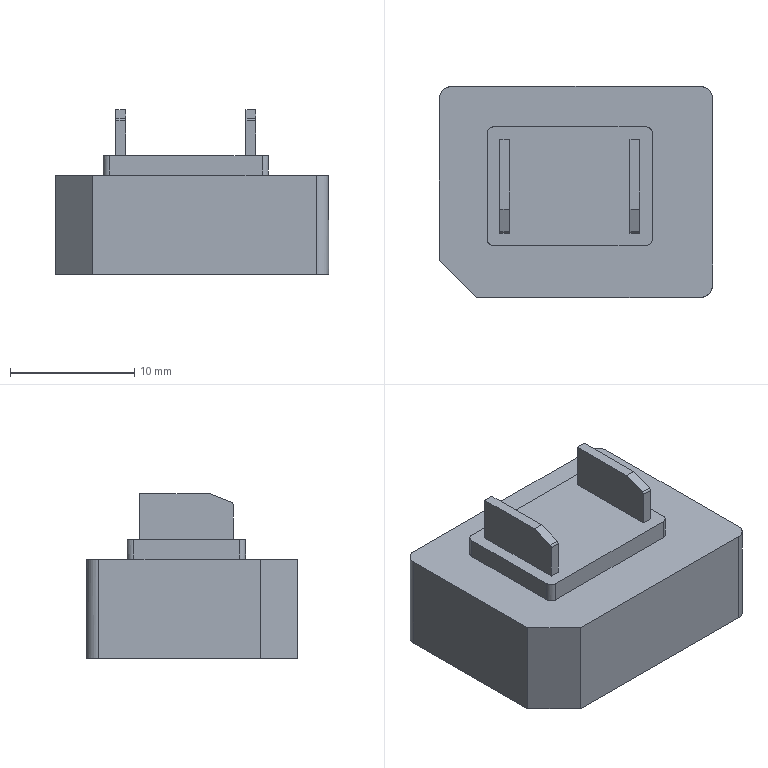NC program | PowerMill | posted by the shop | part box 22 x 17 x 13.286 mm
Lines 5762 to 6864 of 53717:
( TOOL ID   R1_1_1 )
( TOOL DIA. 2. TIP RAD 1. LENGTH 57.16 )
( Z = -2.154 )
T4 M6
T10
G91 G28 Z0
G0 G90 G54
M08
S18000 M3
X0 Y0 M8
G43 Z10.795 H4
X5.291 Y-4.211
Z-.615
G1 Z-1.815 F1200
X5.286 Y-4.216 Z-1.832 F2000
X5.277 Y-4.225 Z-1.866
X5.212 Y-4.248 Z-1.964
X5.217 Y-4.243 Z-1.927
X5.225 Y-4.235 Z-1.885
X5.236 Y-4.224 Z-1.839
X5.251 Y-4.209 Z-1.789
X5.268 Y-4.192 Z-1.739
X5.286 Y-4.174 Z-1.696
X5.304 Y-4.156 Z-1.66
X5.321 Y-4.139 Z-1.629
X5.336 Y-4.124 Z-1.607
X5.344 Y-4.073 Z-1.516
X5.343 Y-4.074 Z-1.517
X5.316 Y-4.102 Z-1.553
X5.29 Y-4.127 Z-1.593
X5.266 Y-4.151 Z-1.635
X5.244 Y-4.173 Z-1.68
X5.225 Y-4.193 Z-1.728
X5.207 Y-4.21 Z-1.778
X5.192 Y-4.225 Z-1.829
X5.18 Y-4.237 Z-1.882
X5.171 Y-4.247 Z-1.936
X5.164 Y-4.254 Z-1.989
X5.16 Y-4.257 Z-2.042
X5.116 Y-4.26 Z-2.107
Z-2.094
X5.118 Y-4.257 Z-2.035
X5.123 Y-4.252 Z-1.978
X5.13 Y-4.245 Z-1.921
X5.141 Y-4.234 Z-1.864
X5.154 Y-4.221 Z-1.81
X5.17 Y-4.205 Z-1.757
X5.188 Y-4.187 Z-1.706
X5.208 Y-4.167 Z-1.657
X5.231 Y-4.144 Z-1.611
X5.255 Y-4.12 Z-1.568
X5.282 Y-4.093 Z-1.527
X5.31 Y-4.065 Z-1.49
X5.341 Y-4.034 Z-1.455
X5.349 Y-4.026 Z-1.447
X5.355 Y-3.978 Z-1.387
X5.333 Y-3.999 Z-1.405
X5.303 Y-4.03 Z-1.436
X5.274 Y-4.059 Z-1.47
X5.246 Y-4.087 Z-1.508
X5.219 Y-4.114 Z-1.549
X5.194 Y-4.139 Z-1.594
X5.171 Y-4.162 Z-1.642
X5.15 Y-4.183 Z-1.692
X5.131 Y-4.202 Z-1.744
X5.115 Y-4.218 Z-1.798
X5.103 Y-4.23 Z-1.845
X5.093 Y-4.24 Z-1.894
X5.084 Y-4.248 Z-1.943
X5.079 Y-4.254 Z-1.994
X5.075 Y-4.258 Z-2.044
X5.073 Y-4.26 Z-2.095
Z-2.133
X5.031 Z-2.138
Z-2.096
X5.033 Y-4.258 Z-2.04
X5.037 Y-4.253 Z-1.984
X5.044 Y-4.246 Z-1.928
X5.054 Y-4.236 Z-1.874
X5.067 Y-4.224 Z-1.819
X5.082 Y-4.208 Z-1.765
X5.101 Y-4.19 Z-1.71
X5.122 Y-4.168 Z-1.656
X5.145 Y-4.146 Z-1.606
X5.169 Y-4.121 Z-1.558
X5.196 Y-4.095 Z-1.513
X5.224 Y-4.066 Z-1.472
X5.254 Y-4.036 Z-1.433
X5.285 Y-4.005 Z-1.399
X5.318 Y-3.972 Z-1.367
X5.352 Y-3.938 Z-1.34
X5.357 Y-3.933 Z-1.336
X5.355 Y-3.893 Z-1.295
X5.337 Y-3.91 Z-1.306
X5.307 Y-3.941 Z-1.329
X5.276 Y-3.972 Z-1.356
X5.244 Y-4.004 Z-1.389
X5.212 Y-4.036 Z-1.426
X5.181 Y-4.067 Z-1.468
X5.153 Y-4.095 Z-1.511
X5.128 Y-4.12 Z-1.553
X5.107 Y-4.141 Z-1.596
X5.082 Y-4.166 Z-1.65
X5.06 Y-4.188 Z-1.705
X5.041 Y-4.207 Z-1.76
X5.026 Y-4.222 Z-1.816
X5.013 Y-4.235 Z-1.871
X5.002 Y-4.246 Z-1.927
X4.995 Y-4.253 Z-1.984
X4.99 Y-4.258 Z-2.041
X4.988 Y-4.26 Z-2.097
Z-2.143
X4.946 Z-2.149
Z-2.098
X4.948 Y-4.258 Z-2.041
X4.952 Y-4.253 Z-1.985
X4.959 Y-4.246 Z-1.93
X4.969 Y-4.237 Z-1.876
X4.981 Y-4.224 Z-1.822
X4.996 Y-4.209 Z-1.768
X5.014 Y-4.191 Z-1.716
X5.035 Y-4.171 Z-1.663
X5.058 Y-4.148 Z-1.612
X5.085 Y-4.121 Z-1.557
X5.113 Y-4.092 Z-1.507
X5.143 Y-4.062 Z-1.46
X5.174 Y-4.031 Z-1.417
X5.206 Y-3.999 Z-1.378
X5.239 Y-3.967 Z-1.343
X5.272 Y-3.933 Z-1.313
X5.306 Y-3.9 Z-1.287
X5.339 Y-3.866 Z-1.265
X5.356 Y-3.85 Z-1.256
Y-3.807 Z-1.219
X5.34 Y-3.823 Z-1.227
X5.306 Y-3.857 Z-1.247
X5.272 Y-3.892 Z-1.272
X5.237 Y-3.926 Z-1.301
X5.202 Y-3.961 Z-1.334
X5.167 Y-3.996 Z-1.372
X5.133 Y-4.03 Z-1.415
X5.1 Y-4.063 Z-1.461
X5.069 Y-4.094 Z-1.511
X5.04 Y-4.123 Z-1.561
X5.014 Y-4.149 Z-1.612
X4.992 Y-4.171 Z-1.661
X4.974 Y-4.189 Z-1.708
X4.958 Y-4.205 Z-1.755
X4.942 Y-4.221 Z-1.81
X4.929 Y-4.234 Z-1.866
X4.918 Y-4.245 Z-1.923
X4.911 Y-4.253 Z-1.98
X4.906 Y-4.257 Z-2.038
X4.904 Y-4.26 Z-2.096
Z-2.153
X4.861
Z-2.099
X4.863 Y-4.258 Z-2.042
X4.867 Y-4.253 Z-1.986
X4.875 Y-4.246 Z-1.929
X4.885 Y-4.236 Z-1.874
X4.898 Y-4.223 Z-1.818
X4.913 Y-4.207 Z-1.763
X4.932 Y-4.189 Z-1.708
X4.953 Y-4.167 Z-1.654
X4.978 Y-4.143 Z-1.6
X5.005 Y-4.115 Z-1.547
X5.036 Y-4.085 Z-1.495
X5.069 Y-4.052 Z-1.444
X5.105 Y-4.015 Z-1.395
X5.138 Y-3.983 Z-1.355
X5.173 Y-3.948 Z-1.317
X5.209 Y-3.912 Z-1.283
X5.246 Y-3.875 Z-1.252
X5.283 Y-3.837 Z-1.226
X5.32 Y-3.8 Z-1.204
X5.356 Y-3.765 Z-1.187
X5.354 Y-3.724 Z-1.16
X5.322 Y-3.756 Z-1.173
X5.286 Y-3.792 Z-1.19
X5.25 Y-3.828 Z-1.213
X5.214 Y-3.865 Z-1.24
X5.176 Y-3.902 Z-1.272
X5.138 Y-3.94 Z-1.308
X5.1 Y-3.978 Z-1.35
X5.063 Y-4.016 Z-1.396
X5.026 Y-4.052 Z-1.446
X4.993 Y-4.085 Z-1.495
X4.963 Y-4.115 Z-1.546
X4.936 Y-4.142 Z-1.598
X4.912 Y-4.167 Z-1.651
X4.89 Y-4.188 Z-1.705
X4.871 Y-4.207 Z-1.76
X4.856 Y-4.223 Z-1.815
X4.843 Y-4.236 Z-1.871
X4.833 Y-4.246 Z-1.927
X4.825 Y-4.253 Z-1.984
X4.821 Y-4.258 Z-2.04
X4.819 Y-4.26 Z-2.097
Z-2.153
X4.776
Z-2.094
X4.778 Y-4.257 Z-2.037
X4.783 Y-4.253 Z-1.98
X4.79 Y-4.245 Z-1.924
X4.801 Y-4.235 Z-1.869
X4.814 Y-4.222 Z-1.814
X4.829 Y-4.207 Z-1.76
X4.847 Y-4.188 Z-1.707
X4.869 Y-4.167 Z-1.653
X4.893 Y-4.143 Z-1.6
X4.92 Y-4.115 Z-1.547
X4.95 Y-4.085 Z-1.496
X4.984 Y-4.052 Z-1.446
X5.02 Y-4.016 Z-1.397
X5.059 Y-3.977 Z-1.349
X5.1 Y-3.935 Z-1.304
X5.14 Y-3.895 Z-1.264
X5.179 Y-3.856 Z-1.23
X5.218 Y-3.818 Z-1.202
X5.255 Y-3.781 Z-1.177
X5.292 Y-3.744 Z-1.158
X5.329 Y-3.707 Z-1.142
X5.352 Y-3.683 Z-1.134
X5.353 Y-3.64 Z-1.11
X5.35 Y-3.644 Z-1.111
X5.323 Y-3.67 Z-1.119
X5.295 Y-3.698 Z-1.129
X5.262 Y-3.731 Z-1.145
X5.223 Y-3.771 Z-1.167
X5.189 Y-3.804 Z-1.189
X5.162 Y-3.831 Z-1.208
X5.139 Y-3.854 Z-1.227
X5.108 Y-3.885 Z-1.254
X5.062 Y-3.931 Z-1.299
X5.02 Y-3.974 Z-1.346
X4.98 Y-4.013 Z-1.393
X4.944 Y-4.049 Z-1.442
X4.911 Y-4.083 Z-1.492
X4.88 Y-4.113 Z-1.543
X4.853 Y-4.141 Z-1.595
X4.828 Y-4.165 Z-1.648
X4.806 Y-4.187 Z-1.702
X4.788 Y-4.206 Z-1.757
X4.772 Y-4.222 Z-1.812
X4.759 Y-4.235 Z-1.868
X4.748 Y-4.245 Z-1.924
X4.741 Y-4.253 Z-1.98
X4.736 Y-4.257 Z-2.037
X4.734 Y-4.26 Z-2.095
Z-2.153
X4.691
Z-2.095
X4.693 Y-4.257 Z-2.038
X4.698 Y-4.253 Z-1.981
X4.706 Y-4.245 Z-1.925
X4.716 Y-4.235 Z-1.869
X4.729 Y-4.222 Z-1.813
X4.745 Y-4.206 Z-1.758
X4.764 Y-4.187 Z-1.703
X4.785 Y-4.166 Z-1.649
X4.81 Y-4.141 Z-1.596
X4.838 Y-4.113 Z-1.543
X4.862 Y-4.089 Z-1.501
X4.886 Y-4.064 Z-1.463
X4.915 Y-4.036 Z-1.423
X4.947 Y-4.003 Z-1.381
X4.985 Y-3.966 Z-1.337
X5.027 Y-3.924 Z-1.292
X5.071 Y-3.879 Z-1.25
X5.116 Y-3.835 Z-1.211
X5.159 Y-3.792 Z-1.179
X5.2 Y-3.751 Z-1.152
X5.239 Y-3.712 Z-1.129
X5.276 Y-3.675 Z-1.112
X5.31 Y-3.641 Z-1.1
X5.343 Y-3.608 Z-1.091
X5.353 Y-3.598 Z-1.089
X5.352 Y-3.556 Z-1.07
X5.351 Y-3.557
X5.32 Y-3.588 Z-1.076
X5.288 Y-3.621 Z-1.085
X5.25 Y-3.658 Z-1.1
X5.208 Y-3.7 Z-1.12
X5.172 Y-3.736 Z-1.14
X5.142 Y-3.766 Z-1.159
X5.115 Y-3.794 Z-1.18
X5.064 Y-3.845 Z-1.22
X5.016 Y-3.892 Z-1.261
X4.972 Y-3.936 Z-1.305
X4.931 Y-3.978 Z-1.35
X4.893 Y-4.016 Z-1.397
X4.857 Y-4.052 Z-1.445
X4.823 Y-4.085 Z-1.496
X4.793 Y-4.116 Z-1.548
X4.765 Y-4.143 Z-1.601
X4.741 Y-4.168 Z-1.654
X4.72 Y-4.189 Z-1.708
X4.701 Y-4.207 Z-1.762
X4.685 Y-4.223 Z-1.817
X4.673 Y-4.236 Z-1.873
X4.663 Y-4.246 Z-1.928
X4.655 Y-4.253 Z-1.985
X4.651 Y-4.258 Z-2.042
X4.649 Y-4.26 Z-2.099
Z-2.153
X4.607
Z-2.094
X4.609 Y-4.257 Z-2.037
X4.613 Y-4.253 Z-1.98
X4.621 Y-4.245 Z-1.924
X4.631 Y-4.235 Z-1.868
X4.644 Y-4.222 Z-1.812
X4.66 Y-4.206 Z-1.757
X4.679 Y-4.187 Z-1.702
X4.701 Y-4.165 Z-1.649
X4.725 Y-4.141 Z-1.595
X4.753 Y-4.113 Z-1.543
X4.784 Y-4.083 Z-1.491
X4.817 Y-4.049 Z-1.441
X4.843 Y-4.023 Z-1.405
X4.872 Y-3.994 Z-1.369
X4.905 Y-3.961 Z-1.331
X4.944 Y-3.922 Z-1.291
X4.987 Y-3.879 Z-1.25
X5.034 Y-3.832 Z-1.209
X5.083 Y-3.783 Z-1.171
X5.13 Y-3.736 Z-1.139
X5.175 Y-3.691 Z-1.113
X5.217 Y-3.649 Z-1.092
X5.256 Y-3.61 Z-1.075
X5.293 Y-3.573 Z-1.063
X5.327 Y-3.539 Z-1.055
X5.351 Y-3.515 Z-1.052
Y-3.473 Z-1.035
X5.347 Y-3.477
X5.311 Y-3.513 Z-1.041
X5.273 Y-3.551 Z-1.05
X5.233 Y-3.591 Z-1.064
X5.19 Y-3.634 Z-1.082
X5.144 Y-3.68 Z-1.105
X5.096 Y-3.728 Z-1.134
X5.046 Y-3.778 Z-1.168
X4.996 Y-3.828 Z-1.206
X4.949 Y-3.874 Z-1.246
X4.907 Y-3.916 Z-1.285
X4.871 Y-3.953 Z-1.322
X4.838 Y-3.985 Z-1.359
X4.809 Y-4.014 Z-1.394
X4.773 Y-4.05 Z-1.443
X4.74 Y-4.083 Z-1.493
X4.71 Y-4.114 Z-1.544
X4.682 Y-4.141 Z-1.597
X4.658 Y-4.166 Z-1.65
X4.636 Y-4.188 Z-1.705
X4.617 Y-4.206 Z-1.759
X4.601 Y-4.222 Z-1.815
X4.588 Y-4.235 Z-1.871
X4.578 Y-4.246 Z-1.927
X4.571 Y-4.253 Z-1.983
X4.566 Y-4.258 Z-2.039
X4.564 Y-4.26 Z-2.096
Z-2.153
X4.522 Z-2.15
Z-2.094
X4.524 Y-4.257 Z-2.036
X4.529 Y-4.253 Z-1.979
X4.536 Y-4.245 Z-1.923
X4.546 Y-4.235 Z-1.867
X4.559 Y-4.222 Z-1.811
X4.575 Y-4.206 Z-1.757
X4.594 Y-4.187 Z-1.703
X4.616 Y-4.165 Z-1.649
X4.64 Y-4.141 Z-1.596
X4.668 Y-4.113 Z-1.544
X4.699 Y-4.083 Z-1.492
X4.732 Y-4.049 Z-1.441
X4.768 Y-4.013 Z-1.393
X4.807 Y-3.974 Z-1.346
X4.849 Y-3.932 Z-1.301
X4.893 Y-3.888 Z-1.257
X4.941 Y-3.841 Z-1.216
X4.991 Y-3.79 Z-1.177
X5.044 Y-3.737 Z-1.14
X5.101 Y-3.681 Z-1.105
X5.144 Y-3.637 Z-1.082
X5.189 Y-3.592 Z-1.061
X5.236 Y-3.545 Z-1.044
X5.284 Y-3.497 Z-1.031
X5.335 Y-3.447 Z-1.02
X5.351 Y-3.43 Z-1.018
Y-3.388 Z-1.001
X5.348 Y-3.39
X5.299 Y-3.44 Z-1.01
X5.25 Y-3.489 Z-1.022
X5.2 Y-3.538 Z-1.039
X5.15 Y-3.589 Z-1.059
X5.098 Y-3.641 Z-1.084
X5.047 Y-3.692 Z-1.112
X4.996 Y-3.743 Z-1.144
X4.944 Y-3.794 Z-1.18
X4.895 Y-3.844 Z-1.219
X4.848 Y-3.891 Z-1.261
X4.803 Y-3.936 Z-1.304
X4.761 Y-3.978 Z-1.35
X4.722 Y-4.016 Z-1.397
X4.686 Y-4.052 Z-1.446
X4.653 Y-4.086 Z-1.496
X4.623 Y-4.116 Z-1.548
X4.596 Y-4.143 Z-1.601
X4.571 Y-4.168 Z-1.654
X4.55 Y-4.189 Z-1.708
X4.531 Y-4.208 Z-1.762
X4.516 Y-4.223 Z-1.817
X4.503 Y-4.236 Z-1.873
X4.493 Y-4.246 Z-1.929
X4.486 Y-4.253 Z-1.985
X4.481 Y-4.258 Z-2.042
X4.479 Y-4.26 Z-2.099
Z-2.133
X4.437 Z-2.117
Z-2.095
X4.439 Y-4.258 Z-2.039
X4.444 Y-4.253 Z-1.982
X4.451 Y-4.245 Z-1.925
X4.462 Y-4.235 Z-1.868
X4.475 Y-4.221 Z-1.812
X4.491 Y-4.205 Z-1.756
X4.51 Y-4.186 Z-1.701
X4.532 Y-4.165 Z-1.647
X4.556 Y-4.14 Z-1.594
X4.583 Y-4.114 Z-1.544
X4.614 Y-4.083 Z-1.492
X4.647 Y-4.049 Z-1.441
X4.684 Y-4.012 Z-1.392
X4.723 Y-3.973 Z-1.345
X4.763 Y-3.934 Z-1.302
X4.806 Y-3.891 Z-1.26
X4.851 Y-3.845 Z-1.22
X4.9 Y-3.796 Z-1.182
X4.953 Y-3.743 Z-1.145
X5.008 Y-3.688 Z-1.11
X5.066 Y-3.631 Z-1.079
X5.123 Y-3.573 Z-1.051
X5.18 Y-3.516 Z-1.028
X5.235 Y-3.461 Z-1.01
X5.288 Y-3.409 Z-.996
X5.339 Y-3.357 Z-.986
X5.351 Y-3.345 Z-.984
Y-3.303 Z-.967
X5.317 Y-3.336 Z-.973
X5.267 Y-3.387 Z-.984
X5.211 Y-3.442 Z-1.001
X5.149 Y-3.505 Z-1.023
X5.086 Y-3.568 Z-1.049
X5.025 Y-3.629 Z-1.078
X4.968 Y-3.686 Z-1.109
X4.913 Y-3.741 Z-1.143
X4.86 Y-3.793 Z-1.18
X4.811 Y-3.843 Z-1.219
X4.764 Y-3.89 Z-1.26
X4.719 Y-3.935 Z-1.304
X4.677 Y-3.977 Z-1.35
X4.638 Y-4.016 Z-1.397
X4.601 Y-4.052 Z-1.446
X4.568 Y-4.086 Z-1.496
X4.538 Y-4.116 Z-1.548
X4.512 Y-4.142 Z-1.598
X4.488 Y-4.166 Z-1.65
X4.466 Y-4.188 Z-1.704
X4.447 Y-4.207 Z-1.76
X4.431 Y-4.223 Z-1.816
X4.418 Y-4.236 Z-1.872
X4.408 Y-4.246 Z-1.929
X4.401 Y-4.253 Z-1.985
X4.396 Y-4.258 Z-2.041
X4.394 Y-4.26 Z-2.096
Z-2.1
X4.352 Y-4.259 Z-2.084
X4.355 Y-4.257 Z-2.027
X4.36 Y-4.251 Z-1.97
X4.368 Y-4.243 Z-1.914
X4.379 Y-4.233 Z-1.858
X4.392 Y-4.219 Z-1.803
X4.409 Y-4.203 Z-1.747
X4.428 Y-4.183 Z-1.693
X4.45 Y-4.161 Z-1.639
X4.476 Y-4.136 Z-1.586
X4.504 Y-4.108 Z-1.534
X4.535 Y-4.077 Z-1.483
X4.569 Y-4.043 Z-1.433
X4.605 Y-4.006 Z-1.384
X4.645 Y-3.967 Z-1.337
X4.688 Y-3.924 Z-1.292
X4.733 Y-3.878 Z-1.249
X4.781 Y-3.83 Z-1.208
X4.832 Y-3.78 Z-1.169
X4.884 Y-3.727 Z-1.134
X4.939 Y-3.673 Z-1.101
X4.995 Y-3.617 Z-1.072
X5.052 Y-3.56 Z-1.047
X5.111 Y-3.5 Z-1.021
X5.177 Y-3.434 Z-.995
X5.233 Y-3.378 Z-.977
X5.285 Y-3.326 Z-.963
X5.338 Y-3.274 Z-.952
X5.351 Y-3.261 Z-.95
Y-3.218 Z-.933
X5.339 Y-3.23 Z-.935
X5.295 Y-3.274 Z-.943
X5.245 Y-3.324 Z-.956
X5.188 Y-3.381 Z-.975
X5.112 Y-3.457 Z-1.004
X5.049 Y-3.52 Z-1.029
X4.982 Y-3.587 Z-1.058
X4.92 Y-3.649 Z-1.089
X4.864 Y-3.705 Z-1.12
X4.812 Y-3.757 Z-1.153
X4.764 Y-3.805 Z-1.188
X4.719 Y-3.851 Z-1.225
X4.675 Y-3.894 Z-1.263
X4.633 Y-3.936 Z-1.305
X4.593 Y-3.976 Z-1.349
X4.554 Y-4.015 Z-1.395
X4.518 Y-4.051 Z-1.444
X4.485 Y-4.085 Z-1.495
X4.453 Y-4.116 Z-1.548
X4.428 Y-4.141 Z-1.596
X4.405 Y-4.164 Z-1.646
X4.383 Y-4.186 Z-1.7
X4.364 Y-4.205 Z-1.756
X4.348 Y-4.222 Z-1.812
X4.334 Y-4.235 Z-1.867
X4.324 Y-4.245 Z-1.92
X4.318 Y-4.252 Z-1.972
X4.313 Y-4.256 Z-2.022
X4.282 Y-4.245 Z-1.938
X4.289 Y-4.237 Z-1.887
X4.3 Y-4.227 Z-1.835
X4.314 Y-4.213 Z-1.783
X4.33 Y-4.196 Z-1.73
X4.35 Y-4.177 Z-1.676
X4.373 Y-4.154 Z-1.623
X4.399 Y-4.128 Z-1.57
X4.428 Y-4.099 Z-1.518
X4.459 Y-4.067 Z-1.467
X4.49 Y-4.036 Z-1.423
X4.525 Y-4.001 Z-1.378
X4.564 Y-3.962 Z-1.333
X4.608 Y-3.919 Z-1.288
X4.655 Y-3.872 Z-1.243
X4.704 Y-3.822 Z-1.202
X4.753 Y-3.774 Z-1.165
X4.799 Y-3.728 Z-1.134
X4.843 Y-3.683 Z-1.107
X4.895 Y-3.632 Z-1.079
X4.957 Y-3.569 Z-1.05
X5.027 Y-3.5 Z-1.021
X5.087 Y-3.44 Z-.997
X5.142 Y-3.384 Z-.975
X5.192 Y-3.335 Z-.956
X5.238 Y-3.289 Z-.941
X5.285 Y-3.242 Z-.929
X5.332 Y-3.195 Z-.919
X5.351 Y-3.176 Z-.916
Y-3.133 Z-.899
X5.306 Y-3.178 Z-.907
X5.254 Y-3.23 Z-.92
X5.206 Y-3.278 Z-.935
X5.158 Y-3.327 Z-.952
X5.11 Y-3.375 Z-.97
X5.062 Y-3.423 Z-.99
X5.014 Y-3.47 Z-1.009
X4.966 Y-3.518 Z-1.029
X4.918 Y-3.566 Z-1.049
X4.86 Y-3.625 Z-1.076
X4.803 Y-3.681 Z-1.106
X4.748 Y-3.736 Z-1.139
X4.696 Y-3.788 Z-1.175
X4.647 Y-3.837 Z-1.214
X4.599 Y-3.885 Z-1.255
X4.554 Y-3.93 Z-1.298
X4.512 Y-3.972 Z-1.344
X4.472 Y-4.013 Z-1.393
X4.436 Y-4.048 Z-1.441
X4.403 Y-4.081 Z-1.489
X4.374 Y-4.11 Z-1.537
X4.348 Y-4.136 Z-1.586
X4.325 Y-4.16 Z-1.636
X4.304 Y-4.18 Z-1.687
X4.286 Y-4.198 Z-1.738
X4.271 Y-4.213 Z-1.792
X4.258 Y-4.226 Z-1.846
X4.236 Y-4.205 Z-1.779
X4.248 Y-4.194 Z-1.737
X4.262 Y-4.18 Z-1.693
X4.28 Y-4.162 Z-1.646
X4.302 Y-4.14 Z-1.596
X4.328 Y-4.114 Z-1.544
X4.355 Y-4.087 Z-1.498
X4.38 Y-4.061 Z-1.458
X4.406 Y-4.036 Z-1.422
X4.444 Y-3.998 Z-1.373
X4.485 Y-3.957 Z-1.326
X4.529 Y-3.912 Z-1.281
X4.576 Y-3.865 Z-1.238
X4.626 Y-3.816 Z-1.197
X4.677 Y-3.765 Z-1.159
X4.724 Y-3.718 Z-1.128
X4.778 Y-3.664 Z-1.097
X4.832 Y-3.61 Z-1.069
X4.894 Y-3.547 Z-1.04
X4.975 Y-3.467 Z-1.008
X5.035 Y-3.407 Z-.984
X5.105 Y-3.337 Z-.955
X5.161 Y-3.281 Z-.933
X5.215 Y-3.227 Z-.915
X5.27 Y-3.172 Z-.899
X5.317 Y-3.124 Z-.888
X5.351 Y-3.091 Z-.882
Y-3.048 Z-.865
X5.312 Y-3.088 Z-.872
X5.264 Y-3.135 Z-.883
X5.222 Y-3.177 Z-.895
X5.18 Y-3.22 Z-.91
X5.138 Y-3.262 Z-.926
X5.096 Y-3.304 Z-.942
X5.054 Y-3.346 Z-.959
X5.012 Y-3.388 Z-.976
X4.97 Y-3.429 Z-.993
X4.928 Y-3.471 Z-1.01
X4.886 Y-3.513 Z-1.027
X4.844 Y-3.555 Z-1.044
X4.785 Y-3.614 Z-1.071
X4.728 Y-3.672 Z-1.101
X4.673 Y-3.726 Z-1.133
X4.62 Y-3.779 Z-1.169
X4.57 Y-3.829 Z-1.207
X4.522 Y-3.878 Z-1.248
X4.476 Y-3.924 Z-1.292
X4.433 Y-3.967 Z-1.338
X4.394 Y-4.005 Z-1.383
X4.359 Y-4.04 Z-1.429
X4.328 Y-4.072 Z-1.475
X4.3 Y-4.1 Z-1.521
X4.275 Y-4.124 Z-1.568
X4.253 Y-4.146 Z-1.616
X4.234 Y-4.165 Z-1.665
X4.218 Y-4.182 Z-1.714
X4.2 Y-4.157 Z-1.659
X4.214 Y-4.143 Z-1.62
X4.231 Y-4.126 Z-1.581
X4.252 Y-4.105 Z-1.538
X4.278 Y-4.079 Z-1.491
X4.307 Y-4.05 Z-1.444
X4.336 Y-4.021 Z-1.403
X4.361 Y-3.996 Z-1.371
X4.385 Y-3.972 Z-1.343
X4.43 Y-3.927 Z-1.296
X4.477 Y-3.88 Z-1.25
X4.527 Y-3.83 Z-1.208
X4.579 Y-3.778 Z-1.168
X4.632 Y-3.725 Z-1.132
X4.686 Y-3.671 Z-1.1
X4.741 Y-3.616 Z-1.071
X4.796 Y-3.561 Z-1.047
X4.837 Y-3.52 Z-1.03
X4.876 Y-3.481 Z-1.014
X4.914 Y-3.443 Z-.999
X4.952 Y-3.405 Z-.983
X4.99 Y-3.367 Z-.968
X5.028 Y-3.329 Z-.953
X5.066 Y-3.291 Z-.937
X5.104 Y-3.253 Z-.922
X5.142 Y-3.215 Z-.907
X5.18 Y-3.177 Z-.893
X5.218 Y-3.139 Z-.88
X5.256 Y-3.101 Z-.868
X5.296 Y-3.061 Z-.858
X5.335 Y-3.022 Z-.851
X5.351 Y-3.006 Z-.848
Y-2.964 Z-.831
X5.343 Y-2.971 Z-.832
X5.306 Y-3.009 Z-.839
X5.264 Y-3.051 Z-.849
X5.227 Y-3.088 Z-.86
X5.19 Y-3.125 Z-.872
X5.153 Y-3.161 Z-.886
X5.116 Y-3.198 Z-.9
X5.08 Y-3.235 Z-.915
X5.043 Y-3.271 Z-.929
X5.007 Y-3.308 Z-.944
X4.97 Y-3.344 Z-.959
X4.934 Y-3.381 Z-.974
X4.897 Y-3.418 Z-.989
X4.859 Y-3.456 Z-1.004
X4.819 Y-3.496 Z-1.02
X4.777 Y-3.537 Z-1.037
X4.733 Y-3.581 Z-1.055
X4.675 Y-3.64 Z-1.084
X4.618 Y-3.696 Z-1.115
X4.565 Y-3.75 Z-1.149
X4.513 Y-3.801 Z-1.185
X4.464 Y-3.851 Z-1.225
X4.426 Y-3.888 Z-1.258
X4.385 Y-3.929 Z-1.297
X4.347 Y-3.967 Z-1.338
X4.313 Y-4.001 Z-1.379
X4.282 Y-4.032 Z-1.421
X4.254 Y-4.06 Z-1.465
X4.228 Y-4.086 Z-1.511
X4.205 Y-4.11 Z-1.558
X4.184 Y-4.131 Z-1.607
X4.166 Y-4.106 Z-1.566
X4.189 Y-4.083 Z-1.517
X4.214 Y-4.058 Z-1.47
X4.242 Y-4.03 Z-1.424
X4.273 Y-3.999 Z-1.38
X4.306 Y-3.966 Z-1.338
X4.343 Y-3.929 Z-1.297
X4.382 Y-3.891 Z-1.259
X4.423 Y-3.849 Z-1.223
X4.472 Y-3.8 Z-1.184
X4.525 Y-3.747 Z-1.147
X4.581 Y-3.691 Z-1.112
X4.638 Y-3.634 Z-1.081
X4.693 Y-3.579 Z-1.054
X4.748 Y-3.524 Z-1.032
X4.912 Y-3.36 Z-.965
X5.077 Y-3.195 Z-.899
X5.131 Y-3.141 Z-.878
X5.185 Y-3.087 Z-.857
X5.239 Y-3.033 Z-.839
X5.286 Y-2.987 Z-.827
X5.344 Y-2.928 Z-.816
X5.351 Y-2.921 Z-.814
Y-2.879 Z-.797
X5.322 Y-2.908 Z-.803
X5.266 Y-2.964 Z-.815
X5.219 Y-3.01 Z-.828
X5.169 Y-3.061 Z-.846
X5.101 Y-3.129 Z-.873
X5.04 Y-3.19 Z-.897
X4.761 Y-3.469 Z-1.009
X4.695 Y-3.534 Z-1.035
X4.633 Y-3.597 Z-1.062
X4.574 Y-3.656 Z-1.092
X4.518 Y-3.712 Z-1.124
X4.465 Y-3.765 Z-1.159
X4.414 Y-3.815 Z-1.196
X4.365 Y-3.864 Z-1.237
X4.331 Y-3.899 Z-1.268
X4.297 Y-3.932 Z-1.302
X4.265 Y-3.965 Z-1.341
X4.233 Y-3.997 Z-1.383
X4.203 Y-4.027 Z-1.429
X4.175 Y-4.055 Z-1.477
X4.15 Y-4.08 Z-1.526
X4.145 Y-4.042 Z-1.469
X4.171 Y-4.016 Z-1.423
X4.2 Y-3.988 Z-1.379
X4.23 Y-3.957 Z-1.337
X4.263 Y-3.925 Z-1.298
X4.298 Y-3.889 Z-1.26
X4.336 Y-3.851 Z-1.225
X4.377 Y-3.811 Z-1.192
X4.414 Y-3.773 Z-1.165
X4.464 Y-3.723 Z-1.131
X4.516 Y-3.672 Z-1.101
X4.568 Y-3.619 Z-1.073
X4.621 Y-3.566 Z-1.048
X4.675 Y-3.513 Z-1.026
X4.828 Y-3.359 Z-.964
X5.02 Y-3.167 Z-.889
X5.103 Y-3.085 Z-.855
X5.164 Y-3.023 Z-.831
X5.213 Y-2.974 Z-.813
X5.26 Y-2.928 Z-.8
X5.313 Y-2.874 Z-.788
X5.351 Y-2.836 Z-.78
Y-2.794 Z-.763
X5.335 Y-2.81 Z-.766
X5.281 Y-2.864 Z-.777
X5.235 Y-2.91 Z-.79
X5.18 Y-2.965 Z-.808
X5.117 Y-3.028 Z-.833
X4.988 Y-3.157 Z-.884
X4.858 Y-3.287 Z-.936
X4.747 Y-3.398 Z-.98
X4.628 Y-3.517 Z-1.028
X4.566 Y-3.579 Z-1.054
X4.507 Y-3.638 Z-1.082
X4.45 Y-3.694 Z-1.114
X4.396 Y-3.749 Z-1.148
X4.344 Y-3.801 Z-1.185
X4.306 Y-3.839 Z-1.216
X4.27 Y-3.875 Z-1.25
X4.235 Y-3.91 Z-1.286
X4.203 Y-3.942 Z-1.326
X4.171 Y-3.973 Z-1.37
X4.142 Y-4.003 Z-1.416
X4.14 Y-3.962 Z-1.368
X4.164 Y-3.939 Z-1.332
X4.19 Y-3.913 Z-1.299
X4.221 Y-3.882 Z-1.263
X4.257 Y-3.846 Z-1.226
X4.292 Y-3.81 Z-1.194
X4.324 Y-3.778 Z-1.169
X4.355 Y-3.747 Z-1.147
X4.402 Y-3.7 Z-1.117
X4.451 Y-3.652 Z-1.09
X4.5 Y-3.603 Z-1.065
X4.549 Y-3.553 Z-1.043
X4.599 Y-3.503 Z-1.023
X4.938 Y-3.164 Z-.887
X5.124 Y-2.979 Z-.813
X5.173 Y-2.929 Z-.793
X5.223 Y-2.88 Z-.776
X5.267 Y-2.835 Z-.764
X5.315 Y-2.787 Z-.753
X5.351 Y-2.752 Z-.746
Y-2.709 Z-.729
X5.305 Y-2.755 Z-.738
X5.26 Y-2.8 Z-.749
X5.215 Y-2.845 Z-.762
X5.164 Y-2.896 Z-.78
X5.113 Y-2.947 Z-.8
X4.836 Y-3.224 Z-.911
X4.559 Y-3.501 Z-1.021
X4.534 Y-3.526 Z-1.032
X4.508 Y-3.552 Z-1.043
X4.482 Y-3.577 Z-1.054
X4.444 Y-3.616 Z-1.071
X4.409 Y-3.651 Z-1.089
X4.383 Y-3.677 Z-1.103
X4.359 Y-3.701 Z-1.117
X4.334 Y-3.726 Z-1.134
X4.304 Y-3.756 Z-1.155
X4.274 Y-3.786 Z-1.178
X4.244 Y-3.816 Z-1.203
X4.216 Y-3.844 Z-1.23
X4.189 Y-3.871 Z-1.26
X4.163 Y-3.897 Z-1.291
X4.138 Y-3.922 Z-1.324
X4.135 Y-3.882 Z-1.285
X4.161 Y-3.857 Z-1.254
X4.187 Y-3.83 Z-1.224
X4.215 Y-3.803 Z-1.197
X4.244 Y-3.774 Z-1.171
X4.274 Y-3.744 Z-1.148
X4.304 Y-3.713 Z-1.127
X4.327 Y-3.691 Z-1.112
X4.35 Y-3.667 Z-1.098
X4.374 Y-3.644 Z-1.085
X4.401 Y-3.617 Z-1.072
X4.44 Y-3.577 Z-1.054
X4.474 Y-3.543 Z-1.039
X4.499 Y-3.519 Z-1.029
X4.523 Y-3.495 Z-1.019
X5.069 Y-2.949 Z-.801
X5.12 Y-2.898 Z-.78
X5.168 Y-2.85 Z-.762
X5.216 Y-2.802 Z-.745
X5.26 Y-2.758 Z-.732
X5.306 Y-2.712 Z-.721
X5.351 Y-2.667 Z-.713
Y-2.624 Z-.695
X5.304 Y-2.671 Z-.705
X5.251 Y-2.724 Z-.717
X5.205 Y-2.77 Z-.731
X5.156 Y-2.819 Z-.749
X5.081 Y-2.894 Z-.779
X4.785 Y-3.19 Z-.897
X4.489 Y-3.486 Z-1.016
X4.426 Y-3.549 Z-1.041
X4.372 Y-3.603 Z-1.065
X4.325 Y-3.65 Z-1.089
X4.283 Y-3.692 Z-1.115
X4.245 Y-3.73 Z-1.142
X4.215 Y-3.761 Z-1.167
X4.181 Y-3.794 Z-1.199
X4.136 Y-3.839 Z-1.246
Y-3.796 Z-1.212
X4.159 Y-3.773 Z-1.187
X4.188 Y-3.744 Z-1.161
X4.223 Y-3.71 Z-1.132
X4.259 Y-3.674 Z-1.106
X4.298 Y-3.635 Z-1.082
X4.342 Y-3.591 Z-1.059
X4.392 Y-3.54 Z-1.037
X4.452 Y-3.481 Z-1.014
X5.114 Y-2.818 Z-.749
X5.161 Y-2.772 Z-.73
X5.208 Y-2.725 Z-.713
X5.248 Y-2.685 Z-.701
X5.3 Y-2.633 Z-.688
X5.34 Y-2.593 Z-.68
X5.351 Y-2.582 Z-.679
Y-2.539 Z-.661
X5.327 Y-2.564 Z-.666
X5.29 Y-2.6 Z-.674
X5.254 Y-2.637 Z-.684
X5.212 Y-2.678 Z-.696
X5.176 Y-2.714 Z-.707
X5.14 Y-2.75 Z-.721
X4.926 Y-2.964 Z-.807
X4.382 Y-3.508 Z-1.025
X4.334 Y-3.556 Z-1.044
X4.29 Y-3.6 Z-1.065
X4.251 Y-3.639 Z-1.088
X4.216 Y-3.675 Z-1.112
X4.18 Y-3.711 Z-1.142
X4.138 Y-3.752 Z-1.179
X4.14 Y-3.708 Z-1.148
X4.171 Y-3.677 Z-1.122
X4.206 Y-3.642 Z-1.096
X4.247 Y-3.6 Z-1.07
X4.282 Y-3.566 Z-1.05
X4.323 Y-3.525 Z-1.032
X4.379 Y-3.469 Z-1.009
X4.466 Y-3.382 Z-.974
X5.119 Y-2.729 Z-.713
X5.166 Y-2.682 Z-.694
X5.214 Y-2.634 Z-.677
X5.253 Y-2.595 Z-.666
X5.291 Y-2.557 Z-.656
X5.333 Y-2.514 Z-.647
X5.351 Y-2.497 Z-.645
Y-2.454 Z-.627
X5.33 Y-2.475 Z-.631
X5.293 Y-2.513 Z-.64
X5.255 Y-2.55 Z-.65
X5.212 Y-2.593 Z-.662
X5.175 Y-2.63 Z-.674
X5.138 Y-2.667 Z-.687
X5.001 Y-2.805 Z-.743
X4.529 Y-3.276 Z-.932
X4.393 Y-3.412 Z-.986
X4.323 Y-3.483 Z-1.015
X4.268 Y-3.537 Z-1.041
X4.222 Y-3.584 Z-1.065
X4.197 Y-3.609 Z-1.081
X4.173 Y-3.633 Z-1.099
X4.139 Y-3.667 Z-1.125
Y-3.624 Z-1.102
X4.188 Y-3.575 Z-1.068
X4.222 Y-3.541 Z-1.046
X4.257 Y-3.506 Z-1.028
X4.292 Y-3.471 Z-1.011
X4.327 Y-3.436 Z-.996
X4.363 Y-3.4 Z-.981
X4.913 Y-2.85 Z-.761
X5.143 Y-2.62 Z-.669
X5.178 Y-2.585 Z-.656
X5.214 Y-2.549 Z-.644
X5.254 Y-2.509 Z-.633
X5.29 Y-2.473 Z-.623
X5.326 Y-2.436 Z-.615
X5.351 Y-2.412 Z-.61
Y-2.37 Z-.593
X5.317 Y-2.404 Z-.599
X5.266 Y-2.454 Z-.611
X5.222 Y-2.499 Z-.624
X5.178 Y-2.543 Z-.639
X5.134 Y-2.586 Z-.656
X5.09 Y-2.63 Z-.673
X4.417 Y-3.303 Z-.943
X4.338 Y-3.383 Z-.975
X4.281 Y-3.439 Z-.999
X4.234 Y-3.487 Z-1.023
X4.202 Y-3.519 Z-1.041
X4.167 Y-3.553 Z-1.061
X4.14 Y-3.58 Z-1.08
X4.141 Y-3.537 Z-1.061
X4.18 Y-3.498 Z-1.036
X4.229 Y-3.449 Z-1.009
X4.269 Y-3.409 Z-.988
X4.316 Y-3.362 Z-.966
X4.364 Y-3.314 Z-.947
X4.411 Y-3.267 Z-.928
X5.103 Y-2.575 Z-.651
X5.151 Y-2.527 Z-.632
X5.199 Y-2.479 Z-.614
X5.242 Y-2.436 Z-.601
X5.295 Y-2.383 Z-.587
X5.34 Y-2.339 Z-.578
X5.351 Y-2.327 Z-.577
Y-2.285 Z-.56
X5.341 Y-2.294 Z-.561
X5.302 Y-2.334 Z-.568
X5.251 Y-2.385 Z-.581
X5.212 Y-2.424 Z-.593
X5.164 Y-2.471 Z-.61
X5.117 Y-2.519 Z-.629
X4.427 Y-3.209 Z-.905
X4.381 Y-3.254 Z-.923
X4.336 Y-3.3 Z-.941
X4.291 Y-3.345 Z-.961
X4.246 Y-3.39 Z-.983
X4.19 Y-3.446 Z-1.013
X4.141 Y-3.494 Z-1.043
Y-3.452 Z-1.026
X4.203 Y-3.39 Z-.99
X4.266 Y-3.327 Z-.958
X4.329 Y-3.264 Z-.928
X4.393 Y-3.2 Z-.901
X4.458 Y-3.136 Z-.875
X4.728 Y-2.865 Z-.767
X4.999 Y-2.594 Z-.659
X5.128 Y-2.466 Z-.608
X5.18 Y-2.414 Z-.587
X5.232 Y-2.361 Z-.57
X5.278 Y-2.315 Z-.557
X5.329 Y-2.264 Z-.547
X5.351 Y-2.242 Z-.543
Y-2.2 Z-.526
X5.342 Y-2.209 Z-.527
X5.301 Y-2.25 Z-.536
X5.261 Y-2.29 Z-.546
X5.214 Y-2.337 Z-.56
X5.174 Y-2.377 Z-.573
X5.135 Y-2.416 Z-.587
X4.945 Y-2.606 Z-.664
X4.453 Y-3.098 Z-.86
X4.389 Y-3.161 Z-.885
X4.326 Y-3.224 Z-.912
X4.264 Y-3.287 Z-.941
X4.202 Y-3.349 Z-.974
X4.141 Y-3.41 Z-1.009
Y-3.367 Z-.992
X4.182 Y-3.326 Z-.967
X4.215 Y-3.293 Z-.948
X4.277 Y-3.232 Z-.917
X4.348 Y-3.161 Z-.886
X4.436 Y-3.072 Z-.85
X4.956 Y-2.553 Z-.642
X5.141 Y-2.367 Z-.567
X5.176 Y-2.332 Z-.554
X5.212 Y-2.296 Z-.543
X5.253 Y-2.256 Z-.531
X5.289 Y-2.219 Z-.522
X5.325 Y-2.183 Z-.513
X5.351 Y-2.158 Z-.508
Y-2.115 Z-.492
X5.341 Y-2.125 Z-.493
X5.288 Y-2.178 Z-.504
X5.24 Y-2.226 Z-.516
X5.186 Y-2.28 Z-.534
X5.132 Y-2.334 Z-.555
X4.95 Y-2.516 Z-.628
X4.651 Y-2.815 Z-.747
X4.35 Y-3.116 Z-.868
X4.309 Y-3.157 Z-.885
X4.268 Y-3.198 Z-.905
X4.221 Y-3.245 Z-.929
X4.181 Y-3.285 Z-.951
X4.141 Y-3.325 Z-.975
Y-3.282 Z-.959
X4.185 Y-3.238 Z-.932
X4.23 Y-3.194 Z-.908
X4.275 Y-3.149 Z-.885
X4.32 Y-3.104 Z-.863
X4.366 Y-3.058 Z-.844
X4.904 Y-2.519 Z-.629
X5.142 Y-2.282 Z-.533
X5.177 Y-2.246 Z-.52
X5.213 Y-2.21 Z-.509
X5.254 Y-2.17 Z-.497
X5.29 Y-2.134 Z-.488
X5.326 Y-2.097 Z-.479
X5.35 Y-2.073 Z-.475
Y-2.031 Z-.458
X5.335 Y-2.046 Z-.46
X5.298 Y-2.084 Z-.469
X5.26 Y-2.121 Z-.478
X5.217 Y-2.164 Z-.491
X5.18 Y-2.201 Z-.502
X5.144 Y-2.238 Z-.516
X4.924 Y-2.457 Z-.604
X4.369 Y-3.012 Z-.826
X4.323 Y-3.058 Z-.845
X4.277 Y-3.104 Z-.867
X4.231 Y-3.15 Z-.89
X4.186 Y-3.195 Z-.915
X4.141 Y-3.24 Z-.942
Y-3.197 Z-.925
X4.187 Y-3.152 Z-.897
X4.233 Y-3.106 Z-.872
X4.279 Y-3.06 Z-.849
X4.326 Y-3.013 Z-.827
X4.373 Y-2.966 Z-.807
X5.023 Y-2.315 Z-.547
X5.145 Y-2.194 Z-.498
X5.188 Y-2.15 Z-.482
X5.232 Y-2.106 Z-.469
X5.277 Y-2.062 Z-.456
X5.321 Y-2.018 Z-.446
X5.349 Y-1.99 Z-.441
X5.338 Y-1.958 Z-.426
X5.326 Y-1.971 Z-.428
X5.265 Y-2.031 Z-.442
X5.204 Y-2.092 Z-.46
X5.145 Y-2.152 Z-.482